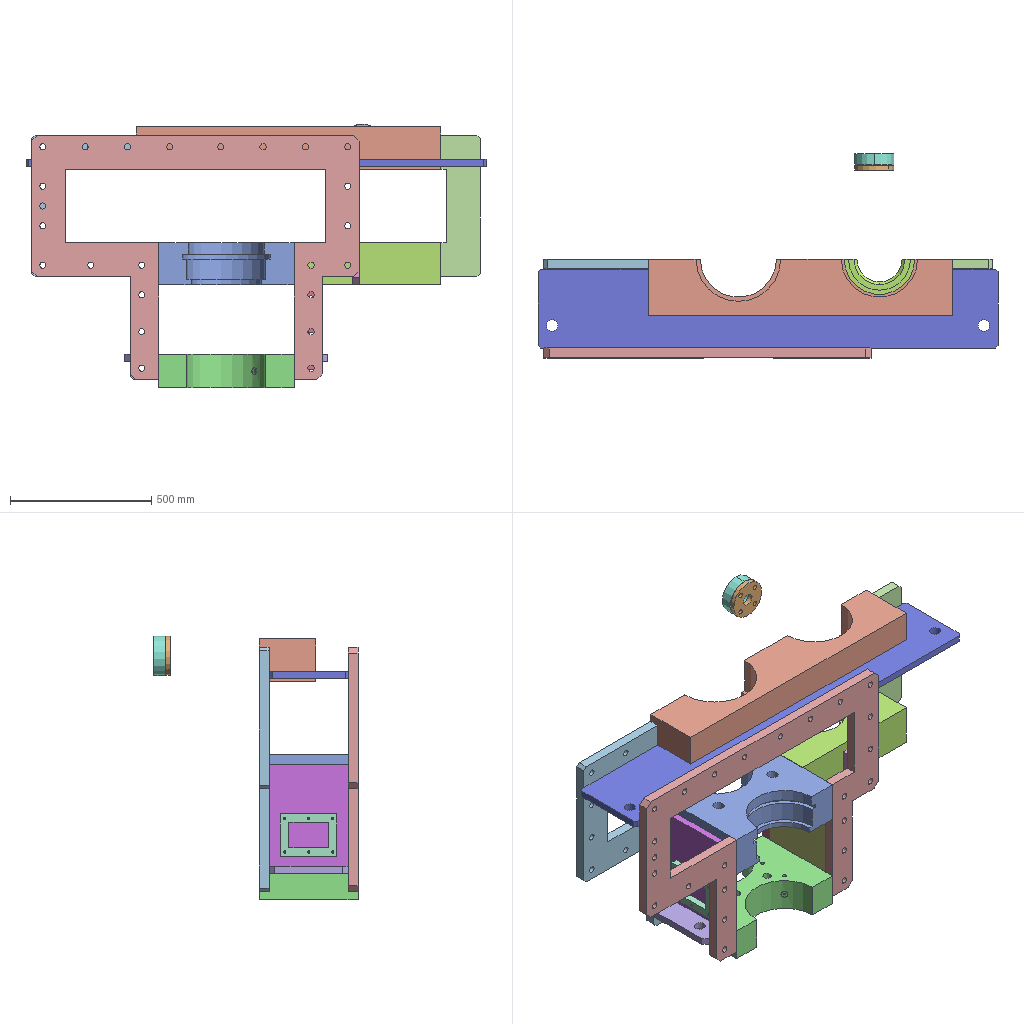Assembly | SolidWorks | 17 different items | 19 placed | box 1630 x 723 x 935 mm
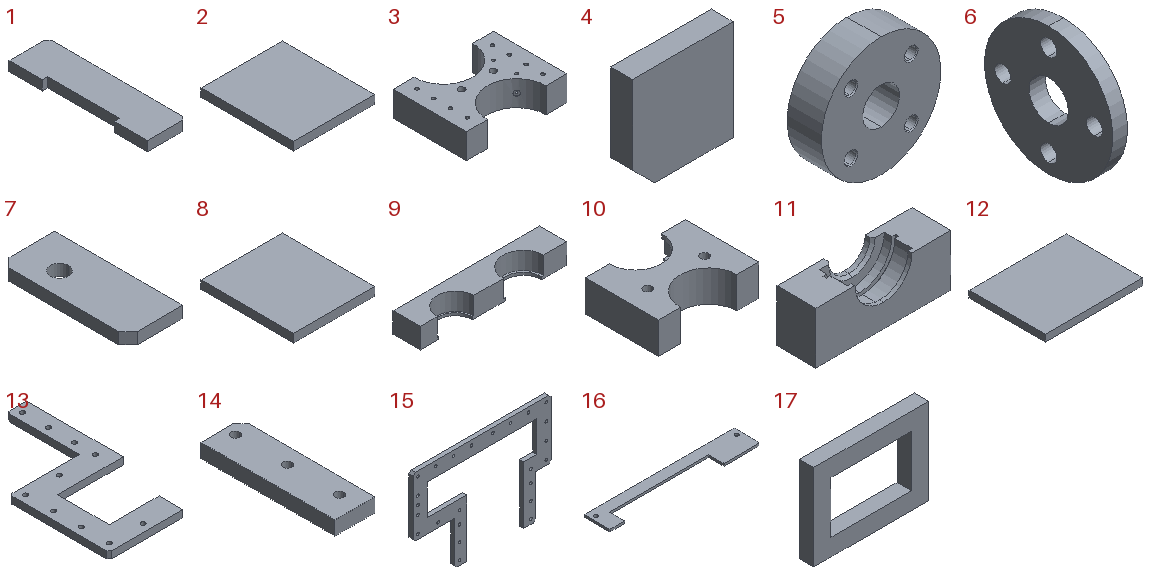Parts list (item | quantity | size | volume | features):
1 | x1 | 140 x 500 x 35 mm | 2262960 mm3 | features Chamfer 1, Extrusion 1
2 | x1 | 245 x 280 x 25 mm | 1715000 mm3 | features Extrusion 1
3 | x1 | 480 x 350 x 120 mm | 12537769 mm3 | features ICE 4, HoleWzd 3, Extrusion 1, MirrorPattern 1
4 | x1 | 115 x 25 x 115 mm | 322812 mm3 | features Extrusion 1
5 | x1 | 140 x 40 x 140 mm | 521515 mm3 | features HoleWzd 2, Extrusion 1
6 | x1 | 18 x 140 x 140 mm | 214823 mm3 | features ICE 1, Revolution 1
7 | x2 | 120 x 280 x 25 mm | 798584 mm3 | features Chamfer 1, Extrusion 1, ICE 1
8 | x1 | 245 x 280 x 25 mm | 1715000 mm3 | features Extrusion 1
9 | x1 | 1080 x 200 x 150 mm | 23020382 mm3 | features ICE 2, RefAxis 2, Extrusion 1
10 | x1 | 480 x 350 x 150 mm | 16005972 mm3 | features ICE 2, Extrusion 1, RevCut 1
11 | x1 | 520 x 150 x 200 mm | 12315251 mm3 | features Chamfer 1, Extrusion 1, HoleWzd 1, RevCut 1
12 | x1 | 360 x 280 x 25 mm | 2520000 mm3 | features Extrusion 1
13 | x1 | 450 x 865 x 35 mm | 5672894 mm3 | features Chamfer 1, Extrusion 1, ICE 1
14 | x1 | 100 x 335 x 35 mm | 1125586 mm3 | features Chamfer 1, Extrusion 1, ICE 1
15 | x1 | 1160 x 35 x 865 mm | 12105689 mm3 | features ICE 2, Chamfer 1, Extrusion 1
16 | x1 | 1630 x 280 x 25 mm | 6887168 mm3 | features Chamfer 1, Extrusion 1, ICE 1
17 | x2 | 200 x 25 x 150 mm | 430967 mm3 | features Extrusion 1, HoleWzd 1, ICE 1
Mates (type | each side: item.copy, entity, surface, feature):
Width | 3.1 face plane Boss-Extrude1 | 3.1 face plane Boss-Extrude1 | 15.1 face plane Boss-Extrude1 | 15.1 face plane Boss-Extrude1
Coincident | 15.1 face plane Boss-Extrude1 | 3.1 face plane Boss-Extrude1
DistanceDim | 15.1 face plane Boss-Extrude1 | 3.1 face plane Boss-Extrude1
Coincident | 15.1 face plane Boss-Extrude1 | 10.1 face plane Boss-Extrude1
Width | 15.1 face plane Boss-Extrude1 | 15.1 face plane Boss-Extrude1 | 10.1 face plane Boss-Extrude1 | 10.1 face plane Boss-Extrude1
Coincident | 15.1 face plane Cut-Extrude1 | 10.1 face plane Boss-Extrude1
Coincident | 3.1 face plane Boss-Extrude1 | 14.1 face plane Boss-Extrude1 | 2 times
Parallel | 3.1 face plane Boss-Extrude1 | 14.1 face plane Boss-Extrude1
DistanceDim | 3.1 face plane Boss-Extrude1 | 14.1 face plane Boss-Extrude1
Coincident | 11.1 face plane Boss-Extrude1 | 14.1 face plane Boss-Extrude1 | 2 times
Coincident | 10.1 face plane Boss-Extrude1 | 11.1 face plane Boss-Extrude1
Coincident | 3.1 face plane Boss-Extrude1 | 13.1 face plane Boss-Extrude1 | 2 times
Parallel | 3.1 face plane Boss-Extrude1 | 13.1 face plane Boss-Extrude1
DistanceDim | 3.1 face plane Boss-Extrude1 | 13.1 face plane Boss-Extrude1
Coincident | 11.1 face plane Boss-Extrude1 | 4.1 face plane Boss-Extrude1 | 2 times
Parallel | 15.1 face plane Boss-Extrude1 | 4.1 face plane Boss-Extrude1
Coincident | 11.1 face plane Boss-Extrude1 | 2.1 face plane Boss-Extrude1
Coincident | 15.1 face plane Boss-Extrude1 | 2.1 face plane Boss-Extrude1
Coincident | 2.1 face plane Boss-Extrude1 | 15.1 select_type:24
Coincident | 3.1 face plane Boss-Extrude1 | 12.1 face plane Boss-Extrude1
Coincident | 13.1 face plane Boss-Extrude1 | 12.1 face plane Boss-Extrude1
DistanceDim | 12.1 face plane Boss-Extrude1 | 3.1 face plane Boss-Extrude1
Coincident | 12.1 face plane Boss-Extrude1 | 17.1 face plane Boss-Extrude1
DistanceDim | 17.1 face plane Boss-Extrude1 | 12.1 face plane Boss-Extrude1
DistanceDim | 13.1 face plane Boss-Extrude1 | 17.1 face plane Boss-Extrude1
DistanceDim | 9.1 face plane Boss-Extrude1 | 13.1 face plane Boss-Extrude1
Coincident | 13.1 face plane Boss-Extrude1 | 9.1 face plane Boss-Extrude1 | 2 times
Coincident | 9.1 face plane Boss-Extrude1 | 16.1 face plane Boss-Extrude1 | 2 times
DistanceDim | 16.1 face plane Boss-Extrude1 | 9.1 face plane Boss-Extrude1
Concentric | 5.1 face cylinder M16 Threaded Hole3 | 6.1 face cylinder Cut-Extrude1
Concentric | 5.1 face cylinder Boss-Extrude1 | 6.1 face cylinder Revolve1
Coincident | 5.1 face plane Boss-Extrude1 | 6.1 face plane Revolve1
Coincident | 11.1 face plane Boss-Extrude1 | 1.1 face plane Boss-Extrude1
Coincident | 9.1 face plane Boss-Extrude1 | 1.1 face plane Boss-Extrude1
DistanceDim | 9.1 axis | 1.1 face plane Boss-Extrude1
Coincident | 7.1 face plane Boss-Extrude1 | 13.1 face plane Boss-Extrude1
Coincident | 7.1 face plane Boss-Extrude1 | 3.1 face plane Boss-Extrude1
Coincident | 7.1 face plane Boss-Extrude1 | 12.1 face plane Boss-Extrude1
Coincident | 3.1 face plane Boss-Extrude1 | 7.2 face plane Boss-Extrude1
Coincident | 14.1 face plane Boss-Extrude1 | 7.2 face plane Boss-Extrude1
Coincident | 2.1 face plane Boss-Extrude1 | 7.2 face plane Boss-Extrude1